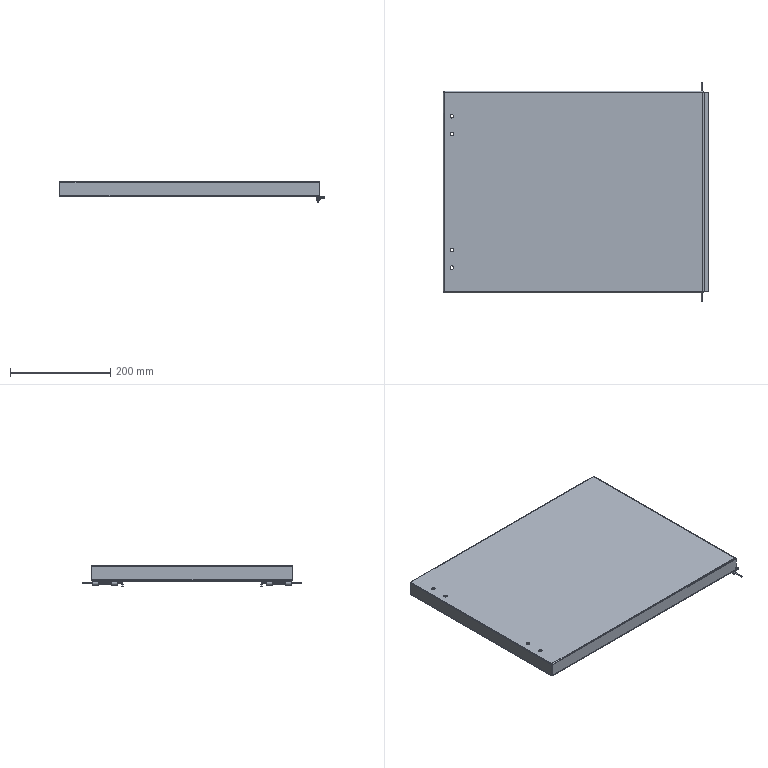Part | 5 solids | 145 faces | box 529.8 x 438.127 x 41 mm | volume 339131 mm3 | plane 76 | cylinder 51 | spline 14 | torus 4 | commonest cylinder face diameters 7 x11 1.473 x8 3 x8 3.6 x8 3.873 x8 7.6 x8